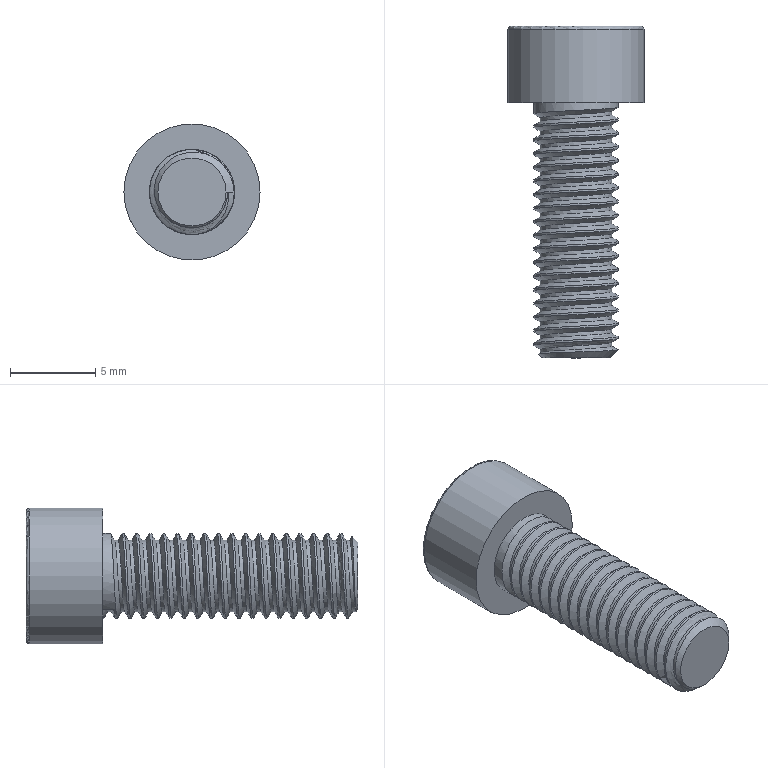Part | STEP file | Tube feed_id962_x_t | 1 solid | 27 faces | box 8 x 19.5 x 8 mm | volume 429.516 mm3 | plane 12 | cylinder 9 | spline 3 | cone 2 | torus 1 | commonest cylinder face diameters 0.4 x6 4.2 x1 5 x1 8 x1